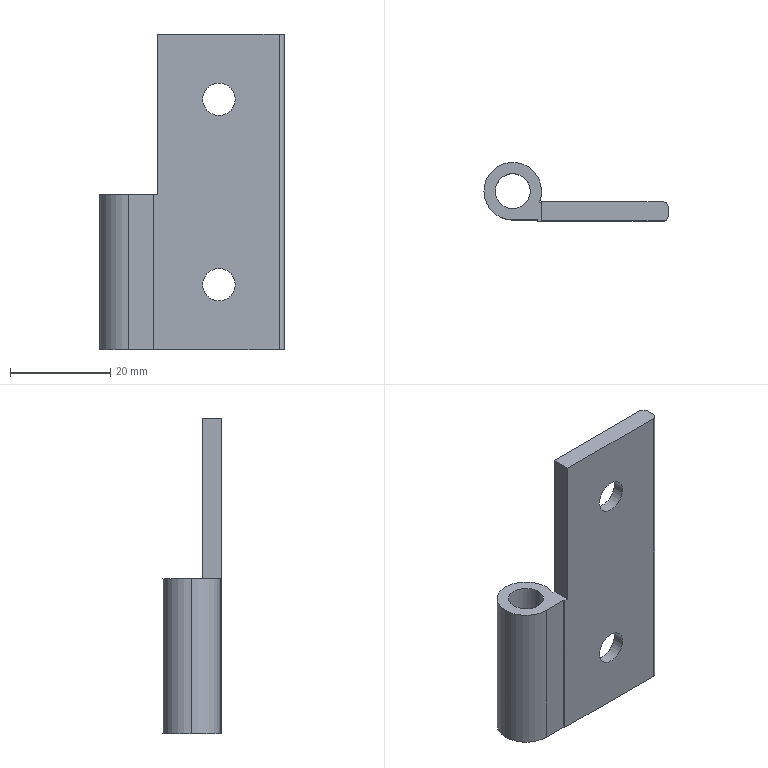Part | NX | features BREP 1 | 1 solid | 26 faces | box 36.75 x 11.75 x 63 mm | volume 7823 mm3 | cylinder 15 | plane 11 | commonest cylinder face diameters 6.5 x4 11 x4 11.5 x3 2 x2 7 x2
STEP:
#1=CARTESIAN_POINT('',(23.5,-3.7,18.5));
#2=VERTEX_POINT('',#1);
#3=CARTESIAN_POINT('',(12.5,-3.7,18.5));
#4=VERTEX_POINT('',#3);
#5=CARTESIAN_POINT('',(18.,-3.7,18.5));
#6=DIRECTION('',(0.,1.,0.));
#7=DIRECTION('',(-1.,0.,0.));
#8=AXIS2_PLACEMENT_3D('',#5,#6,#7);
#9=CIRCLE('',#8,5.5);
#10=EDGE_CURVE('',#2,#4,#9,.T.);
#11=ORIENTED_EDGE('',*,*,#10,.F.);
#12=CARTESIAN_POINT('',(23.5,-2.2,18.5));
#13=VERTEX_POINT('',#12);
#14=CARTESIAN_POINT('',(23.5,-3.7,18.5));
#15=DIRECTION('',(0.,1.,0.));
#16=VECTOR('',#15,1000.);
#17=LINE('',#14,#16);
#18=EDGE_CURVE('',#2,#13,#17,.T.);
#19=ORIENTED_EDGE('',*,*,#18,.T.);
#20=CARTESIAN_POINT('',(12.5,-2.2,18.5));
#21=VERTEX_POINT('',#20);
#22=CARTESIAN_POINT('',(18.,-2.2,18.5));
#23=DIRECTION('',(0.,1.,0.));
#24=DIRECTION('',(-1.,0.,0.));
#25=AXIS2_PLACEMENT_3D('',#22,#23,#24);
#26=CIRCLE('',#25,5.5);
#27=EDGE_CURVE('',#13,#21,#26,.T.);
#28=ORIENTED_EDGE('',*,*,#27,.T.);
#29=CARTESIAN_POINT('',(12.5,-3.7,18.5));
#30=DIRECTION('',(0.,1.,0.));
#31=VECTOR('',#30,1000.);
#32=LINE('',#29,#31);
#33=EDGE_CURVE('',#4,#21,#32,.T.);
#34=ORIENTED_EDGE('',*,*,#33,.F.);
#35=EDGE_LOOP('',(#11,#19,#28,#34));
#36=FACE_BOUND('',#35,.T.);
#37=CARTESIAN_POINT('',(18.,-3.7,18.5));
#38=DIRECTION('',(0.,1.,0.));
#39=DIRECTION('',(-1.,0.,0.));
#40=AXIS2_PLACEMENT_3D('',#37,#38,#39);
#41=CYLINDRICAL_SURFACE('',#40,5.5);
#42=ADVANCED_FACE('',(#36),#41,.F.);
#43=CARTESIAN_POINT('',(23.5,-3.7,-18.5));
#44=VERTEX_POINT('',#43);
#45=CARTESIAN_POINT('',(12.5,-3.7,-18.5));
#46=VERTEX_POINT('',#45);
#47=CARTESIAN_POINT('',(18.,-3.7,-18.5));
#48=DIRECTION('',(0.,1.,0.));
#49=DIRECTION('',(-1.,0.,0.));
#50=AXIS2_PLACEMENT_3D('',#47,#48,#49);
#51=CIRCLE('',#50,5.5);
#52=EDGE_CURVE('',#44,#46,#51,.T.);
#53=ORIENTED_EDGE('',*,*,#52,.F.);
#54=CARTESIAN_POINT('',(23.5,-2.2,-18.5));
#55=VERTEX_POINT('',#54);
#56=CARTESIAN_POINT('',(23.5,-3.7,-18.5));
#57=DIRECTION('',(0.,1.,0.));
#58=VECTOR('',#57,1000.);
#59=LINE('',#56,#58);
#60=EDGE_CURVE('',#44,#55,#59,.T.);
#61=ORIENTED_EDGE('',*,*,#60,.T.);
#62=CARTESIAN_POINT('',(12.5,-2.2,-18.5));
#63=VERTEX_POINT('',#62);
#64=CARTESIAN_POINT('',(18.,-2.2,-18.5));
#65=DIRECTION('',(0.,1.,0.));
#66=DIRECTION('',(-1.,0.,0.));
#67=AXIS2_PLACEMENT_3D('',#64,#65,#66);
#68=CIRCLE('',#67,5.5);
#69=EDGE_CURVE('',#55,#63,#68,.T.);
#70=ORIENTED_EDGE('',*,*,#69,.T.);
#71=CARTESIAN_POINT('',(12.5,-3.7,-18.5));
#72=DIRECTION('',(0.,1.,0.));
#73=VECTOR('',#72,1000.);
#74=LINE('',#71,#73);
#75=EDGE_CURVE('',#46,#63,#74,.T.);
#76=ORIENTED_EDGE('',*,*,#75,.F.);
#77=EDGE_LOOP('',(#53,#61,#70,#76));
#78=FACE_BOUND('',#77,.T.);
#79=CARTESIAN_POINT('',(18.,-3.7,-18.5));
#80=DIRECTION('',(0.,1.,0.));
#81=DIRECTION('',(-1.,0.,0.));
#82=AXIS2_PLACEMENT_3D('',#79,#80,#81);
#83=CYLINDRICAL_SURFACE('',#82,5.5);
#84=ADVANCED_FACE('',(#78),#83,.F.);
#85=CARTESIAN_POINT('',(3.5,0.,-0.5));
#86=VERTEX_POINT('',#85);
#87=CARTESIAN_POINT('',(-3.5,0.,-0.5));
#88=VERTEX_POINT('',#87);
#89=CARTESIAN_POINT('',(0.,0.,-0.5));
#90=DIRECTION('',(0.,0.,-1.));
#91=DIRECTION('',(-1.,0.,0.));
#92=AXIS2_PLACEMENT_3D('',#89,#90,#91);
#93=CIRCLE('',#92,3.5);
#94=EDGE_CURVE('',#86,#88,#93,.T.);
#95=ORIENTED_EDGE('',*,*,#94,.F.);
#96=CARTESIAN_POINT('',(3.5,0.,-31.5));
#97=VERTEX_POINT('',#96);
#98=CARTESIAN_POINT('',(3.5,0.,31.5));
#99=DIRECTION('',(0.,0.,-1.));
#100=VECTOR('',#99,1000.);
#101=LINE('',#98,#100);
#102=EDGE_CURVE('',#86,#97,#101,.T.);
#103=ORIENTED_EDGE('',*,*,#102,.T.);
#104=CARTESIAN_POINT('',(-3.5,0.,-31.5));
#105=VERTEX_POINT('',#104);
#106=CARTESIAN_POINT('',(0.,0.,-31.5));
#107=DIRECTION('',(0.,0.,1.));
#108=DIRECTION('',(1.,0.,0.));
#109=AXIS2_PLACEMENT_3D('',#106,#107,#108);
#110=CIRCLE('',#109,3.5);
#111=EDGE_CURVE('',#105,#97,#110,.T.);
#112=ORIENTED_EDGE('',*,*,#111,.F.);
#113=CARTESIAN_POINT('',(-3.5,0.,31.5));
#114=DIRECTION('',(0.,0.,-1.));
#115=VECTOR('',#114,1000.);
#116=LINE('',#113,#115);
#117=EDGE_CURVE('',#88,#105,#116,.T.);
#118=ORIENTED_EDGE('',*,*,#117,.F.);
#119=EDGE_LOOP('',(#95,#103,#112,#118));
#120=FACE_BOUND('',#119,.T.);
#121=CARTESIAN_POINT('',(0.,0.,31.5));
#122=DIRECTION('',(0.,0.,-1.));
#123=DIRECTION('',(-1.,0.,0.));
#124=AXIS2_PLACEMENT_3D('',#121,#122,#123);
#125=CYLINDRICAL_SURFACE('',#124,3.5);
#126=ADVANCED_FACE('',(#120),#125,.F.);
#127=CARTESIAN_POINT('',(-5.75,0.,-0.5));
#128=VERTEX_POINT('',#127);
#129=CARTESIAN_POINT('',(5.75,0.,-0.5));
#130=VERTEX_POINT('',#129);
#131=CARTESIAN_POINT('',(0.,0.,-0.5));
#132=DIRECTION('',(0.,0.,-1.));
#133=DIRECTION('',(-1.,0.,0.));
#134=AXIS2_PLACEMENT_3D('',#131,#132,#133);
#135=CIRCLE('',#134,5.75);
#136=EDGE_CURVE('',#128,#130,#135,.T.);
#137=ORIENTED_EDGE('',*,*,#136,.T.);
#138=CARTESIAN_POINT('',(5.75,0.,-31.5));
#139=VERTEX_POINT('',#138);
#140=CARTESIAN_POINT('',(5.75,0.,31.5));
#141=DIRECTION('',(0.,0.,-1.));
#142=VECTOR('',#141,1000.);
#143=LINE('',#140,#142);
#144=EDGE_CURVE('',#130,#139,#143,.T.);
#145=ORIENTED_EDGE('',*,*,#144,.T.);
#146=CARTESIAN_POINT('',(-5.75,0.,-31.5));
#147=VERTEX_POINT('',#146);
#148=CARTESIAN_POINT('',(0.,0.,-31.5));
#149=DIRECTION('',(0.,0.,1.));
#150=DIRECTION('',(1.,0.,0.));
#151=AXIS2_PLACEMENT_3D('',#148,#149,#150);
#152=CIRCLE('',#151,5.75);
#153=EDGE_CURVE('',#139,#147,#152,.T.);
#154=ORIENTED_EDGE('',*,*,#153,.T.);
#155=CARTESIAN_POINT('',(-5.75,0.,31.5));
#156=DIRECTION('',(0.,0.,-1.));
#157=VECTOR('',#156,1000.);
#158=LINE('',#155,#157);
#159=EDGE_CURVE('',#128,#147,#158,.T.);
#160=ORIENTED_EDGE('',*,*,#159,.F.);
#161=EDGE_LOOP('',(#137,#145,#154,#160));
#162=FACE_BOUND('',#161,.T.);
#163=CARTESIAN_POINT('',(0.,0.,31.5));
#164=DIRECTION('',(0.,0.,-1.));
#165=DIRECTION('',(-1.,0.,0.));
#166=AXIS2_PLACEMENT_3D('',#163,#164,#165);
#167=CYLINDRICAL_SURFACE('',#166,5.75);
#168=ADVANCED_FACE('',(#162),#167,.T.);
#169=CARTESIAN_POINT('',(0.,-5.75,-0.5));
#170=VERTEX_POINT('',#169);
#171=CARTESIAN_POINT('',(0.,0.,-0.5));
#172=DIRECTION('',(0.,0.,-1.));
#173=DIRECTION('',(-1.,0.,0.));
#174=AXIS2_PLACEMENT_3D('',#171,#172,#173);
#175=CIRCLE('',#174,5.75);
#176=EDGE_CURVE('',#170,#128,#175,.T.);
#177=ORIENTED_EDGE('',*,*,#176,.T.);
#178=ORIENTED_EDGE('',*,*,#159,.T.);
#179=CARTESIAN_POINT('',(0.,-5.75,-31.5));
#180=VERTEX_POINT('',#179);
#181=CARTESIAN_POINT('',(0.,0.,-31.5));
#182=DIRECTION('',(0.,0.,1.));
#183=DIRECTION('',(1.,0.,0.));
#184=AXIS2_PLACEMENT_3D('',#181,#182,#183);
#185=CIRCLE('',#184,5.75);
#186=EDGE_CURVE('',#147,#180,#185,.T.);
#187=ORIENTED_EDGE('',*,*,#186,.T.);
#188=CARTESIAN_POINT('',(0.,-5.75,31.5));
#189=DIRECTION('',(0.,0.,-1.));
#190=VECTOR('',#189,1000.);
#191=LINE('',#188,#190);
#192=EDGE_CURVE('',#170,#180,#191,.T.);
#193=ORIENTED_EDGE('',*,*,#192,.F.);
#194=EDGE_LOOP('',(#177,#178,#187,#193));
#195=FACE_BOUND('',#194,.T.);
#196=CARTESIAN_POINT('',(0.,0.,31.5));
#197=DIRECTION('',(0.,0.,-1.));
#198=DIRECTION('',(-1.,0.,0.));
#199=AXIS2_PLACEMENT_3D('',#196,#197,#198);
#200=CYLINDRICAL_SURFACE('',#199,5.75);
#201=ADVANCED_FACE('',(#195),#200,.T.);
#202=CARTESIAN_POINT('',(21.25,-6.,-18.5));
#203=VERTEX_POINT('',#202);
#204=CARTESIAN_POINT('',(14.75,-6.,-18.5));
#205=VERTEX_POINT('',#204);
#206=CARTESIAN_POINT('',(18.,-6.,-18.5));
#207=DIRECTION('',(0.,1.,0.));
#208=DIRECTION('',(-1.,0.,0.));
#209=AXIS2_PLACEMENT_3D('',#206,#207,#208);
#210=CIRCLE('',#209,3.25);
#211=EDGE_CURVE('',#203,#205,#210,.T.);
#212=ORIENTED_EDGE('',*,*,#211,.F.);
#213=CARTESIAN_POINT('',(21.25,-3.7,-18.5));
#214=VERTEX_POINT('',#213);
#215=CARTESIAN_POINT('',(21.25,-6.,-18.5));
#216=DIRECTION('',(0.,1.,0.));
#217=VECTOR('',#216,1000.);
#218=LINE('',#215,#217);
#219=EDGE_CURVE('',#203,#214,#218,.T.);
#220=ORIENTED_EDGE('',*,*,#219,.T.);
#221=CARTESIAN_POINT('',(14.75,-3.7,-18.5));
#222=VERTEX_POINT('',#221);
#223=CARTESIAN_POINT('',(18.,-3.7,-18.5));
#224=DIRECTION('',(0.,-1.,0.));
#225=DIRECTION('',(-1.,0.,0.));
#226=AXIS2_PLACEMENT_3D('',#223,#224,#225);
#227=CIRCLE('',#226,3.25);
#228=EDGE_CURVE('',#222,#214,#227,.T.);
#229=ORIENTED_EDGE('',*,*,#228,.F.);
#230=CARTESIAN_POINT('',(14.75,-6.,-18.5));
#231=DIRECTION('',(0.,1.,0.));
#232=VECTOR('',#231,1000.);
#233=LINE('',#230,#232);
#234=EDGE_CURVE('',#205,#222,#233,.T.);
#235=ORIENTED_EDGE('',*,*,#234,.F.);
#236=EDGE_LOOP('',(#212,#220,#229,#235));
#237=FACE_BOUND('',#236,.T.);
#238=CARTESIAN_POINT('',(18.,-6.,-18.5));
#239=DIRECTION('',(0.,1.,0.));
#240=DIRECTION('',(-1.,0.,0.));
#241=AXIS2_PLACEMENT_3D('',#238,#239,#240);
#242=CYLINDRICAL_SURFACE('',#241,3.25);
#243=ADVANCED_FACE('',(#237),#242,.F.);
#244=CARTESIAN_POINT('',(21.25,-6.,18.5));
#245=VERTEX_POINT('',#244);
#246=CARTESIAN_POINT('',(14.75,-6.,18.5));
#247=VERTEX_POINT('',#246);
#248=CARTESIAN_POINT('',(18.,-6.,18.5));
#249=DIRECTION('',(0.,1.,0.));
#250=DIRECTION('',(-1.,0.,0.));
#251=AXIS2_PLACEMENT_3D('',#248,#249,#250);
#252=CIRCLE('',#251,3.25);
#253=EDGE_CURVE('',#245,#247,#252,.T.);
#254=ORIENTED_EDGE('',*,*,#253,.F.);
#255=CARTESIAN_POINT('',(21.25,-3.7,18.5));
#256=VERTEX_POINT('',#255);
#257=CARTESIAN_POINT('',(21.25,-6.,18.5));
#258=DIRECTION('',(0.,1.,0.));
#259=VECTOR('',#258,1000.);
#260=LINE('',#257,#259);
#261=EDGE_CURVE('',#245,#256,#260,.T.);
#262=ORIENTED_EDGE('',*,*,#261,.T.);
#263=CARTESIAN_POINT('',(14.75,-3.7,18.5));
#264=VERTEX_POINT('',#263);
#265=CARTESIAN_POINT('',(18.,-3.7,18.5));
#266=DIRECTION('',(0.,-1.,0.));
#267=DIRECTION('',(-1.,0.,0.));
#268=AXIS2_PLACEMENT_3D('',#265,#266,#267);
#269=CIRCLE('',#268,3.25);
#270=EDGE_CURVE('',#264,#256,#269,.T.);
#271=ORIENTED_EDGE('',*,*,#270,.F.);
#272=CARTESIAN_POINT('',(14.75,-6.,18.5));
#273=DIRECTION('',(0.,1.,0.));
#274=VECTOR('',#273,1000.);
#275=LINE('',#272,#274);
#276=EDGE_CURVE('',#247,#264,#275,.T.);
#277=ORIENTED_EDGE('',*,*,#276,.F.);
#278=EDGE_LOOP('',(#254,#262,#271,#277));
#279=FACE_BOUND('',#278,.T.);
#280=CARTESIAN_POINT('',(18.,-6.,18.5));
#281=DIRECTION('',(0.,1.,0.));
#282=DIRECTION('',(-1.,0.,0.));
#283=AXIS2_PLACEMENT_3D('',#280,#281,#282);
#284=CYLINDRICAL_SURFACE('',#283,3.25);
#285=ADVANCED_FACE('',(#279),#284,.F.);
#286=ORIENTED_EDGE('',*,*,#261,.F.);
#287=CARTESIAN_POINT('',(18.,-6.,18.5));
#288=DIRECTION('',(0.,1.,0.));
#289=DIRECTION('',(-1.,0.,0.));
#290=AXIS2_PLACEMENT_3D('',#287,#288,#289);
#291=CIRCLE('',#290,3.25);
#292=EDGE_CURVE('',#247,#245,#291,.T.);
#293=ORIENTED_EDGE('',*,*,#292,.F.);
#294=ORIENTED_EDGE('',*,*,#276,.T.);
#295=CARTESIAN_POINT('',(18.,-3.7,18.5));
#296=DIRECTION('',(0.,-1.,0.));
#297=DIRECTION('',(-1.,0.,0.));
#298=AXIS2_PLACEMENT_3D('',#295,#296,#297);
#299=CIRCLE('',#298,3.25);
#300=EDGE_CURVE('',#256,#264,#299,.T.);
#301=ORIENTED_EDGE('',*,*,#300,.F.);
#302=EDGE_LOOP('',(#286,#293,#294,#301));
#303=FACE_BOUND('',#302,.T.);
#304=CARTESIAN_POINT('',(18.,-6.,18.5));
#305=DIRECTION('',(0.,1.,0.));
#306=DIRECTION('',(-1.,0.,0.));
#307=AXIS2_PLACEMENT_3D('',#304,#305,#306);
#308=CYLINDRICAL_SURFACE('',#307,3.25);
#309=ADVANCED_FACE('',(#303),#308,.F.);
#310=ORIENTED_EDGE('',*,*,#219,.F.);
#311=CARTESIAN_POINT('',(18.,-6.,-18.5));
#312=DIRECTION('',(0.,1.,0.));
#313=DIRECTION('',(-1.,0.,0.));
#314=AXIS2_PLACEMENT_3D('',#311,#312,#313);
#315=CIRCLE('',#314,3.25);
#316=EDGE_CURVE('',#205,#203,#315,.T.);
#317=ORIENTED_EDGE('',*,*,#316,.F.);
#318=ORIENTED_EDGE('',*,*,#234,.T.);
#319=CARTESIAN_POINT('',(18.,-3.7,-18.5));
#320=DIRECTION('',(0.,-1.,0.));
#321=DIRECTION('',(-1.,0.,0.));
#322=AXIS2_PLACEMENT_3D('',#319,#320,#321);
#323=CIRCLE('',#322,3.25);
#324=EDGE_CURVE('',#214,#222,#323,.T.);
#325=ORIENTED_EDGE('',*,*,#324,.F.);
#326=EDGE_LOOP('',(#310,#317,#318,#325));
#327=FACE_BOUND('',#326,.T.);
#328=CARTESIAN_POINT('',(18.,-6.,-18.5));
#329=DIRECTION('',(0.,1.,0.));
#330=DIRECTION('',(-1.,0.,0.));
#331=AXIS2_PLACEMENT_3D('',#328,#329,#330);
#332=CYLINDRICAL_SURFACE('',#331,3.25);
#333=ADVANCED_FACE('',(#327),#332,.F.);
#334=ORIENTED_EDGE('',*,*,#144,.F.);
#335=CARTESIAN_POINT('',(5.312,-2.2,-0.5));
#336=VERTEX_POINT('',#335);
#337=CARTESIAN_POINT('',(0.,0.,-0.5));
#338=DIRECTION('',(0.,0.,-1.));
#339=DIRECTION('',(-1.,0.,0.));
#340=AXIS2_PLACEMENT_3D('',#337,#338,#339);
#341=CIRCLE('',#340,5.75);
#342=EDGE_CURVE('',#130,#336,#341,.T.);
#343=ORIENTED_EDGE('',*,*,#342,.T.);
#344=CARTESIAN_POINT('',(5.312,-2.2,-31.5));
#345=VERTEX_POINT('',#344);
#346=CARTESIAN_POINT('',(5.312,-2.2,31.5));
#347=DIRECTION('',(0.,0.,-1.));
#348=VECTOR('',#347,1000.);
#349=LINE('',#346,#348);
#350=EDGE_CURVE('',#336,#345,#349,.T.);
#351=ORIENTED_EDGE('',*,*,#350,.T.);
#352=CARTESIAN_POINT('',(0.,0.,-31.5));
#353=DIRECTION('',(0.,0.,1.));
#354=DIRECTION('',(1.,0.,0.));
#355=AXIS2_PLACEMENT_3D('',#352,#353,#354);
#356=CIRCLE('',#355,5.75);
#357=EDGE_CURVE('',#345,#139,#356,.T.);
#358=ORIENTED_EDGE('',*,*,#357,.T.);
#359=EDGE_LOOP('',(#334,#343,#351,#358));
#360=FACE_BOUND('',#359,.T.);
#361=CARTESIAN_POINT('',(0.,0.,31.5));
#362=DIRECTION('',(0.,0.,-1.));
#363=DIRECTION('',(-1.,0.,0.));
#364=AXIS2_PLACEMENT_3D('',#361,#362,#363);
#365=CYLINDRICAL_SURFACE('',#364,5.75);
#366=ADVANCED_FACE('',(#360),#365,.T.);
#367=CARTESIAN_POINT('',(5.75,-2.2,31.5));
#368=VERTEX_POINT('',#367);
#369=CARTESIAN_POINT('',(5.75,-6.,31.5));
#370=VERTEX_POINT('',#369);
#371=CARTESIAN_POINT('',(5.75,5.75,31.5));
#372=DIRECTION('',(0.,-1.,0.));
#373=VECTOR('',#372,1000.);
#374=LINE('',#371,#373);
#375=EDGE_CURVE('',#368,#370,#374,.T.);
#376=ORIENTED_EDGE('',*,*,#375,.T.);
#377=CARTESIAN_POINT('',(30.,-6.,31.5));
#378=VERTEX_POINT('',#377);
#379=CARTESIAN_POINT('',(5.,-6.,31.5));
#380=DIRECTION('',(1.,0.,0.));
#381=VECTOR('',#380,1000.);
#382=LINE('',#379,#381);
#383=EDGE_CURVE('',#370,#378,#382,.T.);
#384=ORIENTED_EDGE('',*,*,#383,.T.);
#385=CARTESIAN_POINT('',(31.,-5.,31.5));
#386=VERTEX_POINT('',#385);
#387=CARTESIAN_POINT('',(30.,-5.,31.5));
#388=DIRECTION('',(0.,0.,1.));
#389=DIRECTION('',(1.,0.,0.));
#390=AXIS2_PLACEMENT_3D('',#387,#388,#389);
#391=CIRCLE('',#390,1.);
#392=EDGE_CURVE('',#378,#386,#391,.T.);
#393=ORIENTED_EDGE('',*,*,#392,.T.);
#394=CARTESIAN_POINT('',(31.,-3.2,31.5));
#395=VERTEX_POINT('',#394);
#396=CARTESIAN_POINT('',(31.,-6.,31.5));
#397=DIRECTION('',(0.,1.,0.));
#398=VECTOR('',#397,1000.);
#399=LINE('',#396,#398);
#400=EDGE_CURVE('',#386,#395,#399,.T.);
#401=ORIENTED_EDGE('',*,*,#400,.T.);
#402=CARTESIAN_POINT('',(30.,-2.2,31.5));
#403=VERTEX_POINT('',#402);
#404=CARTESIAN_POINT('',(30.,-3.2,31.5));
#405=DIRECTION('',(0.,0.,1.));
#406=DIRECTION('',(1.,0.,0.));
#407=AXIS2_PLACEMENT_3D('',#404,#405,#406);
#408=CIRCLE('',#407,1.);
#409=EDGE_CURVE('',#395,#403,#408,.T.);
#410=ORIENTED_EDGE('',*,*,#409,.T.);
#411=CARTESIAN_POINT('',(31.,-2.2,31.5));
#412=DIRECTION('',(-1.,0.,0.));
#413=VECTOR('',#412,1000.);
#414=LINE('',#411,#413);
#415=EDGE_CURVE('',#403,#368,#414,.T.);
#416=ORIENTED_EDGE('',*,*,#415,.T.);
#417=EDGE_LOOP('',(#376,#384,#393,#401,#410,#416));
#418=FACE_BOUND('',#417,.T.);
#419=CARTESIAN_POINT('',(0.,0.,31.5));
#420=DIRECTION('',(0.,0.,1.));
#421=DIRECTION('',(1.,0.,0.));
#422=AXIS2_PLACEMENT_3D('',#419,#420,#421);
#423=PLANE('',#422);
#424=ADVANCED_FACE('',(#418),#423,.T.);
#425=CARTESIAN_POINT('',(31.,-5.,-31.5));
#426=VERTEX_POINT('',#425);
#427=CARTESIAN_POINT('',(31.,-3.2,-31.5));
#428=VERTEX_POINT('',#427);
#429=CARTESIAN_POINT('',(31.,-6.,-31.5));
#430=DIRECTION('',(0.,1.,0.));
#431=VECTOR('',#430,1000.);
#432=LINE('',#429,#431);
#433=EDGE_CURVE('',#426,#428,#432,.T.);
#434=ORIENTED_EDGE('',*,*,#433,.F.);
#435=CARTESIAN_POINT('',(30.,-6.,-31.5));
#436=VERTEX_POINT('',#435);
#437=CARTESIAN_POINT('',(30.,-5.,-31.5));
#438=DIRECTION('',(0.,0.,-1.));
#439=DIRECTION('',(1.,0.,0.));
#440=AXIS2_PLACEMENT_3D('',#437,#438,#439);
#441=CIRCLE('',#440,1.);
#442=EDGE_CURVE('',#426,#436,#441,.T.);
#443=ORIENTED_EDGE('',*,*,#442,.T.);
#444=CARTESIAN_POINT('',(5.,-6.,-31.5));
#445=VERTEX_POINT('',#444);
#446=CARTESIAN_POINT('',(5.,-6.,-31.5));
#447=DIRECTION('',(1.,0.,0.));
#448=VECTOR('',#447,1000.);
#449=LINE('',#446,#448);
#450=EDGE_CURVE('',#445,#436,#449,.T.);
#451=ORIENTED_EDGE('',*,*,#450,.F.);
#452=CARTESIAN_POINT('',(5.,-5.75,-31.5));
#453=VERTEX_POINT('',#452);
#454=CARTESIAN_POINT('',(5.,-5.75,-31.5));
#455=DIRECTION('',(0.,-1.,0.));
#456=VECTOR('',#455,1000.);
#457=LINE('',#454,#456);
#458=EDGE_CURVE('',#453,#445,#457,.T.);
#459=ORIENTED_EDGE('',*,*,#458,.F.);
#460=CARTESIAN_POINT('',(0.,-5.75,-31.5));
#461=DIRECTION('',(1.,0.,0.));
#462=VECTOR('',#461,1000.);
#463=LINE('',#460,#462);
#464=EDGE_CURVE('',#180,#453,#463,.T.);
#465=ORIENTED_EDGE('',*,*,#464,.F.);
#466=ORIENTED_EDGE('',*,*,#186,.F.);
#467=ORIENTED_EDGE('',*,*,#153,.F.);
#468=ORIENTED_EDGE('',*,*,#357,.F.);
#469=CARTESIAN_POINT('',(30.,-2.2,-31.5));
#470=VERTEX_POINT('',#469);
#471=CARTESIAN_POINT('',(31.,-2.2,-31.5));
#472=DIRECTION('',(-1.,0.,0.));
#473=VECTOR('',#472,1000.);
#474=LINE('',#471,#473);
#475=EDGE_CURVE('',#470,#345,#474,.T.);
#476=ORIENTED_EDGE('',*,*,#475,.F.);
#477=CARTESIAN_POINT('',(30.,-3.2,-31.5));
#478=DIRECTION('',(0.,0.,-1.));
#479=DIRECTION('',(1.,0.,0.));
#480=AXIS2_PLACEMENT_3D('',#477,#478,#479);
#481=CIRCLE('',#480,1.);
#482=EDGE_CURVE('',#470,#428,#481,.T.);
#483=ORIENTED_EDGE('',*,*,#482,.T.);
#484=EDGE_LOOP('',(#434,#443,#451,#459,#465,#466,#467,#468,#476,#483));
#485=FACE_BOUND('',#484,.T.);
#486=ORIENTED_EDGE('',*,*,#111,.T.);
#487=CARTESIAN_POINT('',(0.,0.,-31.5));
#488=DIRECTION('',(0.,0.,1.));
#489=DIRECTION('',(1.,0.,0.));
#490=AXIS2_PLACEMENT_3D('',#487,#488,#489);
#491=CIRCLE('',#490,3.5);
#492=EDGE_CURVE('',#97,#105,#491,.T.);
#493=ORIENTED_EDGE('',*,*,#492,.T.);
#494=EDGE_LOOP('',(#486,#493));
#495=FACE_BOUND('',#494,.T.);
#496=CARTESIAN_POINT('',(0.,0.,-31.5));
#497=DIRECTION('',(0.,0.,1.));
#498=DIRECTION('',(1.,0.,0.));
#499=AXIS2_PLACEMENT_3D('',#496,#497,#498);
#500=PLANE('',#499);
#501=ADVANCED_FACE('',(#485,#495),#500,.F.);
#502=CARTESIAN_POINT('',(5.,-5.75,-0.5));
#503=VERTEX_POINT('',#502);
#504=CARTESIAN_POINT('',(5.,-5.75,31.5));
#505=DIRECTION('',(0.,0.,-1.));
#506=VECTOR('',#505,1000.);
#507=LINE('',#504,#506);
#508=EDGE_CURVE('',#503,#453,#507,.T.);
#509=ORIENTED_EDGE('',*,*,#508,.F.);
#510=CARTESIAN_POINT('',(0.,-5.75,-0.5));
#511=DIRECTION('',(-1.,0.,0.));
#512=VECTOR('',#511,1000.);
#513=LINE('',#510,#512);
#514=EDGE_CURVE('',#503,#170,#513,.T.);
#515=ORIENTED_EDGE('',*,*,#514,.T.);
#516=ORIENTED_EDGE('',*,*,#192,.T.);
#517=ORIENTED_EDGE('',*,*,#464,.T.);
#518=EDGE_LOOP('',(#509,#515,#516,#517));
#519=FACE_BOUND('',#518,.T.);
#520=CARTESIAN_POINT('',(0.,-5.75,31.5));
#521=DIRECTION('',(0.,1.,0.));
#522=DIRECTION('',(1.,0.,0.));
#523=AXIS2_PLACEMENT_3D('',#520,#521,#522);
#524=PLANE('',#523);
#525=ADVANCED_FACE('',(#519),#524,.F.);
#526=CARTESIAN_POINT('',(5.,-6.,-0.5));
#527=VERTEX_POINT('',#526);
#528=CARTESIAN_POINT('',(5.,-6.,31.5));
#529=DIRECTION('',(0.,0.,-1.));
#530=VECTOR('',#529,1000.);
#531=LINE('',#528,#530);
#532=EDGE_CURVE('',#527,#445,#531,.T.);
#533=ORIENTED_EDGE('',*,*,#532,.F.);
#534=CARTESIAN_POINT('',(5.,-5.75,-0.5));
#535=DIRECTION('',(0.,1.,0.));
#536=VECTOR('',#535,1000.);
#537=LINE('',#534,#536);
#538=EDGE_CURVE('',#527,#503,#537,.T.);
#539=ORIENTED_EDGE('',*,*,#538,.T.);
#540=ORIENTED_EDGE('',*,*,#508,.T.);
#541=ORIENTED_EDGE('',*,*,#458,.T.);
#542=EDGE_LOOP('',(#533,#539,#540,#541));
#543=FACE_BOUND('',#542,.T.);
#544=CARTESIAN_POINT('',(5.,-5.75,31.5));
#545=DIRECTION('',(1.,0.,0.));
#546=DIRECTION('',(0.,1.,0.));
#547=AXIS2_PLACEMENT_3D('',#544,#545,#546);
#548=PLANE('',#547);
#549=ADVANCED_FACE('',(#543),#548,.F.);
#550=ORIENTED_EDGE('',*,*,#383,.F.);
#551=CARTESIAN_POINT('',(5.75,-6.,-0.5));
#552=VERTEX_POINT('',#551);
#553=CARTESIAN_POINT('',(5.75,-6.,-0.5));
#554=DIRECTION('',(0.,0.,1.));
#555=VECTOR('',#554,1000.);
#556=LINE('',#553,#555);
#557=EDGE_CURVE('',#552,#370,#556,.T.);
#558=ORIENTED_EDGE('',*,*,#557,.F.);
#559=CARTESIAN_POINT('',(-5.75,-6.,-0.5));
#560=DIRECTION('',(1.,0.,0.));
#561=VECTOR('',#560,1000.);
#562=LINE('',#559,#561);
#563=EDGE_CURVE('',#527,#552,#562,.T.);
#564=ORIENTED_EDGE('',*,*,#563,.F.);
#565=ORIENTED_EDGE('',*,*,#532,.T.);
#566=ORIENTED_EDGE('',*,*,#450,.T.);
#567=CARTESIAN_POINT('',(30.,-6.,31.5));
#568=DIRECTION('',(0.,0.,1.));
#569=VECTOR('',#568,1000.);
#570=LINE('',#567,#569);
#571=EDGE_CURVE('',#436,#378,#570,.T.);
#572=ORIENTED_EDGE('',*,*,#571,.T.);
#573=EDGE_LOOP('',(#550,#558,#564,#565,#566,#572));
#574=FACE_BOUND('',#573,.T.);
#575=ORIENTED_EDGE('',*,*,#292,.T.);
#576=ORIENTED_EDGE('',*,*,#253,.T.);
#577=EDGE_LOOP('',(#575,#576));
#578=FACE_BOUND('',#577,.T.);
#579=ORIENTED_EDGE('',*,*,#316,.T.);
#580=ORIENTED_EDGE('',*,*,#211,.T.);
#581=EDGE_LOOP('',(#579,#580));
#582=FACE_BOUND('',#581,.T.);
#583=CARTESIAN_POINT('',(5.,-6.,31.5));
#584=DIRECTION('',(0.,1.,0.));
#585=DIRECTION('',(1.,0.,0.));
#586=AXIS2_PLACEMENT_3D('',#583,#584,#585);
#587=PLANE('',#586);
#588=ADVANCED_FACE('',(#574,#578,#582),#587,.F.);
#589=ORIENTED_EDGE('',*,*,#400,.F.);
#590=CARTESIAN_POINT('',(31.,-5.,31.5));
#591=DIRECTION('',(0.,0.,-1.));
#592=VECTOR('',#591,1000.);
#593=LINE('',#590,#592);
#594=EDGE_CURVE('',#386,#426,#593,.T.);
#595=ORIENTED_EDGE('',*,*,#594,.T.);
#596=ORIENTED_EDGE('',*,*,#433,.T.);
#597=CARTESIAN_POINT('',(31.,-3.2,31.5));
#598=DIRECTION('',(0.,0.,1.));
#599=VECTOR('',#598,1000.);
#600=LINE('',#597,#599);
#601=EDGE_CURVE('',#428,#395,#600,.T.);
#602=ORIENTED_EDGE('',*,*,#601,.T.);
#603=EDGE_LOOP('',(#589,#595,#596,#602));
#604=FACE_BOUND('',#603,.T.);
#605=CARTESIAN_POINT('',(31.,-6.,31.5));
#606=DIRECTION('',(-1.,0.,0.));
#607=DIRECTION('',(0.,0.,1.));
#608=AXIS2_PLACEMENT_3D('',#605,#606,#607);
#609=PLANE('',#608);
#610=ADVANCED_FACE('',(#604),#609,.F.);
#611=CARTESIAN_POINT('',(5.75,-2.2,-0.5));
#612=VERTEX_POINT('',#611);
#613=CARTESIAN_POINT('',(31.,-2.2,-0.5));
#614=DIRECTION('',(1.,0.,0.));
#615=VECTOR('',#614,1000.);
#616=LINE('',#613,#615);
#617=EDGE_CURVE('',#336,#612,#616,.T.);
#618=ORIENTED_EDGE('',*,*,#617,.T.);
#619=CARTESIAN_POINT('',(5.75,-2.2,31.5));
#620=DIRECTION('',(0.,0.,1.));
#621=VECTOR('',#620,1000.);
#622=LINE('',#619,#621);
#623=EDGE_CURVE('',#612,#368,#622,.T.);
#624=ORIENTED_EDGE('',*,*,#623,.T.);
#625=ORIENTED_EDGE('',*,*,#415,.F.);
#626=CARTESIAN_POINT('',(30.,-2.2,31.5));
#627=DIRECTION('',(0.,0.,-1.));
#628=VECTOR('',#627,1000.);
#629=LINE('',#626,#628);
#630=EDGE_CURVE('',#403,#470,#629,.T.);
#631=ORIENTED_EDGE('',*,*,#630,.T.);
#632=ORIENTED_EDGE('',*,*,#475,.T.);
#633=ORIENTED_EDGE('',*,*,#350,.F.);
#634=EDGE_LOOP('',(#618,#624,#625,#631,#632,#633));
#635=FACE_BOUND('',#634,.T.);
#636=CARTESIAN_POINT('',(18.,-2.2,18.5));
#637=DIRECTION('',(0.,1.,0.));
#638=DIRECTION('',(-1.,0.,0.));
#639=AXIS2_PLACEMENT_3D('',#636,#637,#638);
#640=CIRCLE('',#639,5.5);
#641=EDGE_CURVE('',#21,#13,#640,.T.);
#642=ORIENTED_EDGE('',*,*,#641,.F.);
#643=ORIENTED_EDGE('',*,*,#27,.F.);
#644=EDGE_LOOP('',(#642,#643));
#645=FACE_BOUND('',#644,.T.);
#646=CARTESIAN_POINT('',(18.,-2.2,-18.5));
#647=DIRECTION('',(0.,1.,0.));
#648=DIRECTION('',(-1.,0.,0.));
#649=AXIS2_PLACEMENT_3D('',#646,#647,#648);
#650=CIRCLE('',#649,5.5);
#651=EDGE_CURVE('',#63,#55,#650,.T.);
#652=ORIENTED_EDGE('',*,*,#651,.F.);
#653=ORIENTED_EDGE('',*,*,#69,.F.);
#654=EDGE_LOOP('',(#652,#653));
#655=FACE_BOUND('',#654,.T.);
#656=CARTESIAN_POINT('',(31.,-2.2,31.5));
#657=DIRECTION('',(0.,-1.,0.));
#658=DIRECTION('',(0.,0.,-1.));
#659=AXIS2_PLACEMENT_3D('',#656,#657,#658);
#660=PLANE('',#659);
#661=ADVANCED_FACE('',(#635,#645,#655),#660,.F.);
#662=ORIENTED_EDGE('',*,*,#102,.F.);
#663=CARTESIAN_POINT('',(0.,0.,-0.5));
#664=DIRECTION('',(0.,0.,-1.));
#665=DIRECTION('',(-1.,0.,0.));
#666=AXIS2_PLACEMENT_3D('',#663,#664,#665);
#667=CIRCLE('',#666,3.5);
#668=EDGE_CURVE('',#88,#86,#667,.T.);
#669=ORIENTED_EDGE('',*,*,#668,.F.);
#670=ORIENTED_EDGE('',*,*,#117,.T.);
#671=ORIENTED_EDGE('',*,*,#492,.F.);
#672=EDGE_LOOP('',(#662,#669,#670,#671));
#673=FACE_BOUND('',#672,.T.);
#674=CARTESIAN_POINT('',(0.,0.,31.5));
#675=DIRECTION('',(0.,0.,-1.));
#676=DIRECTION('',(-1.,0.,0.));
#677=AXIS2_PLACEMENT_3D('',#674,#675,#676);
#678=CYLINDRICAL_SURFACE('',#677,3.5);
#679=ADVANCED_FACE('',(#673),#678,.F.);
#680=ORIENTED_EDGE('',*,*,#392,.F.);
#681=ORIENTED_EDGE('',*,*,#571,.F.);
#682=ORIENTED_EDGE('',*,*,#442,.F.);
#683=ORIENTED_EDGE('',*,*,#594,.F.);
#684=EDGE_LOOP('',(#680,#681,#682,#683));
#685=FACE_BOUND('',#684,.T.);
#686=CARTESIAN_POINT('',(30.,-5.,31.5));
#687=DIRECTION('',(0.,0.,-1.));
#688=DIRECTION('',(-1.,0.,0.));
#689=AXIS2_PLACEMENT_3D('',#686,#687,#688);
#690=CYLINDRICAL_SURFACE('',#689,1.);
#691=ADVANCED_FACE('',(#685),#690,.T.);
#692=ORIENTED_EDGE('',*,*,#409,.F.);
#693=ORIENTED_EDGE('',*,*,#601,.F.);
#694=ORIENTED_EDGE('',*,*,#482,.F.);
#695=ORIENTED_EDGE('',*,*,#630,.F.);
#696=EDGE_LOOP('',(#692,#693,#694,#695));
#697=FACE_BOUND('',#696,.T.);
#698=CARTESIAN_POINT('',(30.,-3.2,31.5));
#699=DIRECTION('',(0.,0.,-1.));
#700=DIRECTION('',(-1.,0.,0.));
#701=AXIS2_PLACEMENT_3D('',#698,#699,#700);
#702=CYLINDRICAL_SURFACE('',#701,1.);
#703=ADVANCED_FACE('',(#697),#702,.T.);
#704=CARTESIAN_POINT('',(5.75,5.75,-0.5));
#705=DIRECTION('',(0.,-1.,0.));
#706=VECTOR('',#705,1000.);
#707=LINE('',#704,#706);
#708=EDGE_CURVE('',#612,#552,#707,.T.);
#709=ORIENTED_EDGE('',*,*,#708,.T.);
#710=ORIENTED_EDGE('',*,*,#557,.T.);
#711=ORIENTED_EDGE('',*,*,#375,.F.);
#712=ORIENTED_EDGE('',*,*,#623,.F.);
#713=EDGE_LOOP('',(#709,#710,#711,#712));
#714=FACE_BOUND('',#713,.T.);
#715=CARTESIAN_POINT('',(5.75,5.75,-0.5));
#716=DIRECTION('',(1.,0.,0.));
#717=DIRECTION('',(0.,1.,0.));
#718=AXIS2_PLACEMENT_3D('',#715,#716,#717);
#719=PLANE('',#718);
#720=ADVANCED_FACE('',(#714),#719,.F.);
#721=ORIENTED_EDGE('',*,*,#563,.T.);
#722=ORIENTED_EDGE('',*,*,#708,.F.);
#723=ORIENTED_EDGE('',*,*,#617,.F.);
#724=ORIENTED_EDGE('',*,*,#342,.F.);
#725=ORIENTED_EDGE('',*,*,#136,.F.);
#726=ORIENTED_EDGE('',*,*,#176,.F.);
#727=ORIENTED_EDGE('',*,*,#514,.F.);
#728=ORIENTED_EDGE('',*,*,#538,.F.);
#729=EDGE_LOOP('',(#721,#722,#723,#724,#725,#726,#727,#728));
#730=FACE_BOUND('',#729,.T.);
#731=ORIENTED_EDGE('',*,*,#668,.T.);
#732=ORIENTED_EDGE('',*,*,#94,.T.);
#733=EDGE_LOOP('',(#731,#732));
#734=FACE_BOUND('',#733,.T.);
#735=CARTESIAN_POINT('',(-5.75,5.75,-0.5));
#736=DIRECTION('',(0.,0.,-1.));
#737=DIRECTION('',(0.,-1.,0.));
#738=AXIS2_PLACEMENT_3D('',#735,#736,#737);
#739=PLANE('',#738);
#740=ADVANCED_FACE('',(#730,#734),#739,.F.);
#741=CARTESIAN_POINT('',(18.,-3.7,-18.5));
#742=DIRECTION('',(0.,1.,0.));
#743=DIRECTION('',(-1.,0.,0.));
#744=AXIS2_PLACEMENT_3D('',#741,#742,#743);
#745=CIRCLE('',#744,5.5);
#746=EDGE_CURVE('',#46,#44,#745,.T.);
#747=ORIENTED_EDGE('',*,*,#746,.T.);
#748=ORIENTED_EDGE('',*,*,#52,.T.);
#749=EDGE_LOOP('',(#747,#748));
#750=FACE_BOUND('',#749,.T.);
#751=ORIENTED_EDGE('',*,*,#228,.T.);
#752=ORIENTED_EDGE('',*,*,#324,.T.);
#753=EDGE_LOOP('',(#751,#752));
#754=FACE_BOUND('',#753,.T.);
#755=CARTESIAN_POINT('',(18.,-3.7,-18.5));
#756=DIRECTION('',(0.,1.,0.));
#757=DIRECTION('',(1.,0.,0.));
#758=AXIS2_PLACEMENT_3D('',#755,#756,#757);
#759=PLANE('',#758);
#760=ADVANCED_FACE('',(#750,#754),#759,.T.);
#761=ORIENTED_EDGE('',*,*,#60,.F.);
#762=ORIENTED_EDGE('',*,*,#746,.F.);
#763=ORIENTED_EDGE('',*,*,#75,.T.);
#764=ORIENTED_EDGE('',*,*,#651,.T.);
#765=EDGE_LOOP('',(#761,#762,#763,#764));
#766=FACE_BOUND('',#765,.T.);
#767=CARTESIAN_POINT('',(18.,-3.7,-18.5));
#768=DIRECTION('',(0.,1.,0.));
#769=DIRECTION('',(-1.,0.,0.));
#770=AXIS2_PLACEMENT_3D('',#767,#768,#769);
#771=CYLINDRICAL_SURFACE('',#770,5.5);
#772=ADVANCED_FACE('',(#766),#771,.F.);
#773=CARTESIAN_POINT('',(18.,-3.7,18.5));
#774=DIRECTION('',(0.,1.,0.));
#775=DIRECTION('',(-1.,0.,0.));
#776=AXIS2_PLACEMENT_3D('',#773,#774,#775);
#777=CIRCLE('',#776,5.5);
#778=EDGE_CURVE('',#4,#2,#777,.T.);
#779=ORIENTED_EDGE('',*,*,#778,.T.);
#780=ORIENTED_EDGE('',*,*,#10,.T.);
#781=EDGE_LOOP('',(#779,#780));
#782=FACE_BOUND('',#781,.T.);
#783=ORIENTED_EDGE('',*,*,#270,.T.);
#784=ORIENTED_EDGE('',*,*,#300,.T.);
#785=EDGE_LOOP('',(#783,#784));
#786=FACE_BOUND('',#785,.T.);
#787=CARTESIAN_POINT('',(18.,-3.7,18.5));
#788=DIRECTION('',(0.,1.,0.));
#789=DIRECTION('',(1.,0.,0.));
#790=AXIS2_PLACEMENT_3D('',#787,#788,#789);
#791=PLANE('',#790);
#792=ADVANCED_FACE('',(#782,#786),#791,.T.);
#793=ORIENTED_EDGE('',*,*,#18,.F.);
#794=ORIENTED_EDGE('',*,*,#778,.F.);
#795=ORIENTED_EDGE('',*,*,#33,.T.);
#796=ORIENTED_EDGE('',*,*,#641,.T.);
#797=EDGE_LOOP('',(#793,#794,#795,#796));
#798=FACE_BOUND('',#797,.T.);
#799=CARTESIAN_POINT('',(18.,-3.7,18.5));
#800=DIRECTION('',(0.,1.,0.));
#801=DIRECTION('',(-1.,0.,0.));
#802=AXIS2_PLACEMENT_3D('',#799,#800,#801);
#803=CYLINDRICAL_SURFACE('',#802,5.5);
#804=ADVANCED_FACE('',(#798),#803,.F.);
#805=CLOSED_SHELL('',(#42,#84,#126,#168,#201,#243,#285,#309,#333,#366,#424,#501,#525,#549,#588,#610,#661,#679,#691,#703,#720,#740,#760,#772,#792,#804));
#806=MANIFOLD_SOLID_BREP('',#805);
#807=(LENGTH_UNIT()NAMED_UNIT(*)SI_UNIT(.MILLI.,.METRE.));
#808=UNCERTAINTY_MEASURE_WITH_UNIT(LENGTH_MEASURE(0.00001),#807,'','');
#809=(NAMED_UNIT(*)PLANE_ANGLE_UNIT()SI_UNIT($,.RADIAN.));
#810=(NAMED_UNIT(*)SI_UNIT($,.STERADIAN.)SOLID_ANGLE_UNIT());
#811=(GEOMETRIC_REPRESENTATION_CONTEXT(3)GLOBAL_UNCERTAINTY_ASSIGNED_CONTEXT((#808))GLOBAL_UNIT_ASSIGNED_CONTEXT((#807,#809,#810))REPRESENTATION_CONTEXT('',''));
#812=ADVANCED_BREP_SHAPE_REPRESENTATION('',(#806),#811);